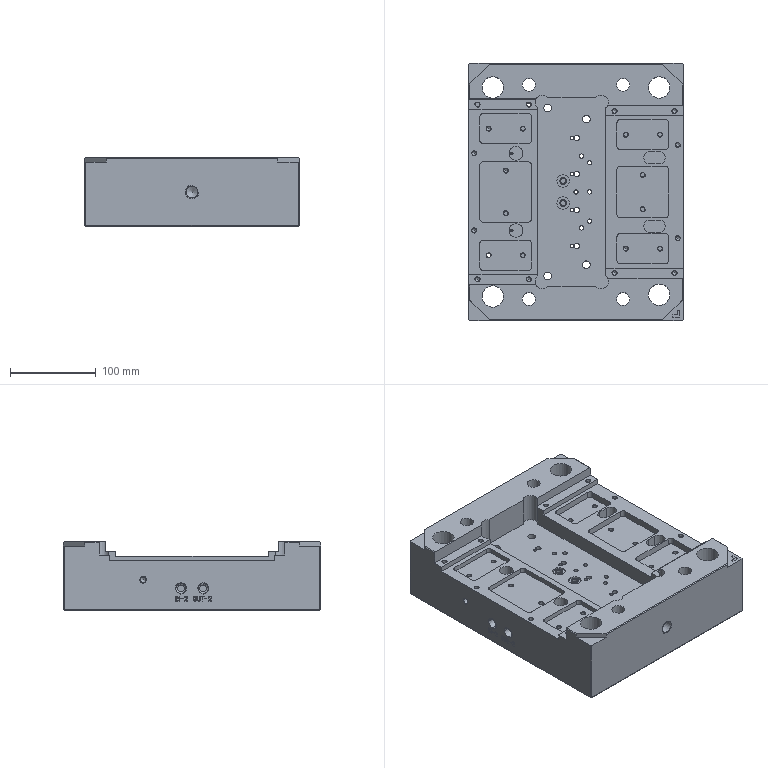NC program | PowerMill | posted with a generic post | part box 250 x 300 x 80 mm
Whole program:
%
O0001
N104 ( POWERMILL CB  : 2026004.0)
N105 ( POST VER      : 2026.0.0.5161)
N106 ( OPTION FILE   : FANUC)
N107 ( OUTPUT WORKPLANE : 1)
N108 (  )
N109 ( TOOL LIST )
N110 (---------------------------------------)
N111 ( NO. | ID        | DIA.| TIP RAD|LENGTH)
N112 (---------------------------------------)
N113 (    1|￠8中心钻_1| 8.0 |  0.0   | 76.0 )
N114 (---------------------------------------)
N115 (  )
N116 ( NUMBER OF TOOLPATHS: 1.0 )
N117 ( ESTIMATED PROGRAM DURATION: 0 HOURS 0 MIN 32 SEC)
N118 (  )
N119 G00 G21 G80 G40 G17
N120 G90
N121 G54
N122 G53 Z0.0
N123 (---------------)
N124 ( START TOOLPATH : 11精光-￠8中心钻-倒角 )
N125 (---------------)
N126 ( TOOL NO.    :1 )
N127 ( TOOL TYPE   : DRILL)
N128 ( TOOL ID     : ￠8中心钻_1)
N129 ( TOOL DIA    : 8.0 LENGTH 76.0)
N130 T1
N131 M6
N132 S4000 M03
N133 G00 G90 X125.0 Y-40.5
N134 G43 Z20.0 H1
N135
N136 G05 P10000 R8
N137 Z0.5
N138 G01 Z-2.5 F480.0
N139 G02 Y-69.5 I0.0 J-14.5 F800.0
N140 G02 Y-40.5 I0.0 J14.5
N141 G00 Z20.0
N142 Y69.5
N143 Z0.5
N144 G01 Z-2.5 F480.0
N145 G02 Y40.5 I0.0 J-14.5 F800.0
N146 G02 Y69.5 I0.0 J14.5
N147 G00 Z20.0
N148 X-125.0
N149 Z0.5
N150 G01 Z-2.5 F480.0
N151 G02 Y40.5 I0.0 J-14.5 F800.0
N152 G02 Y69.5 I0.0 J14.5
N153 G00 Z20.0
N154 Y-40.5
N155 Z0.5
N156 G01 Z-2.5 F480.0
N157 G02 Y-69.5 I0.0 J-14.5 F800.0
N158 G02 Y-40.5 I0.0 J14.5
N159 G00 Z20.0
N160 G05 P0
N161 (---------------)
N162 ( END TOOLPATH : 11精光-￠8中心钻-倒角 )
N163 (---------------)
N164
N165 M05
N166 G53 Z0.0
N167 M30
%